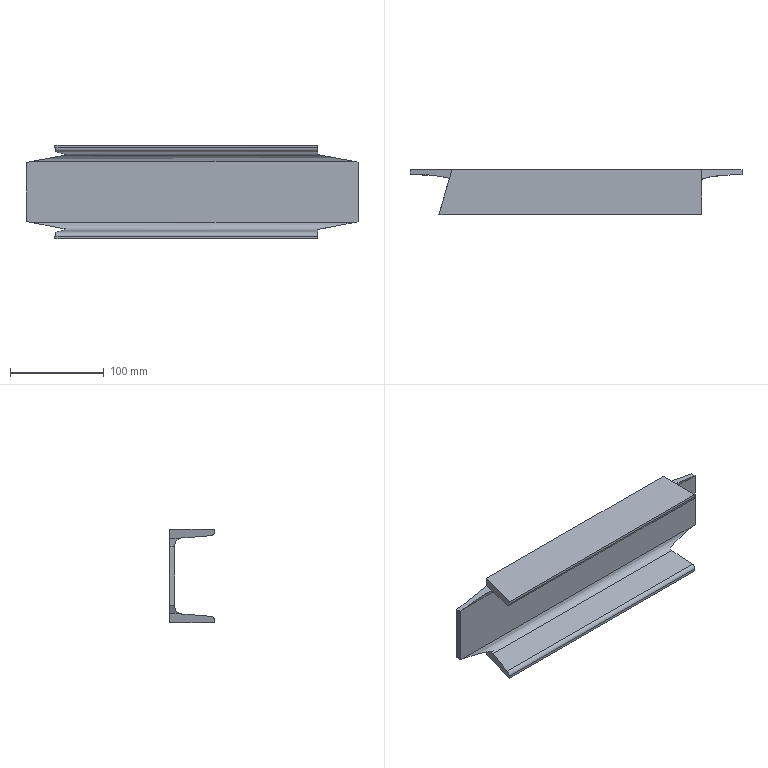Part | STEP file | 11-Channel 100x48_default<machining> | 1 solid | 24 faces | box 355 x 48 x 100 mm | volume 375001 mm3 | plane 20 | cylinder 4 | commonest cylinder face diameters 8.5 x2 17 x2